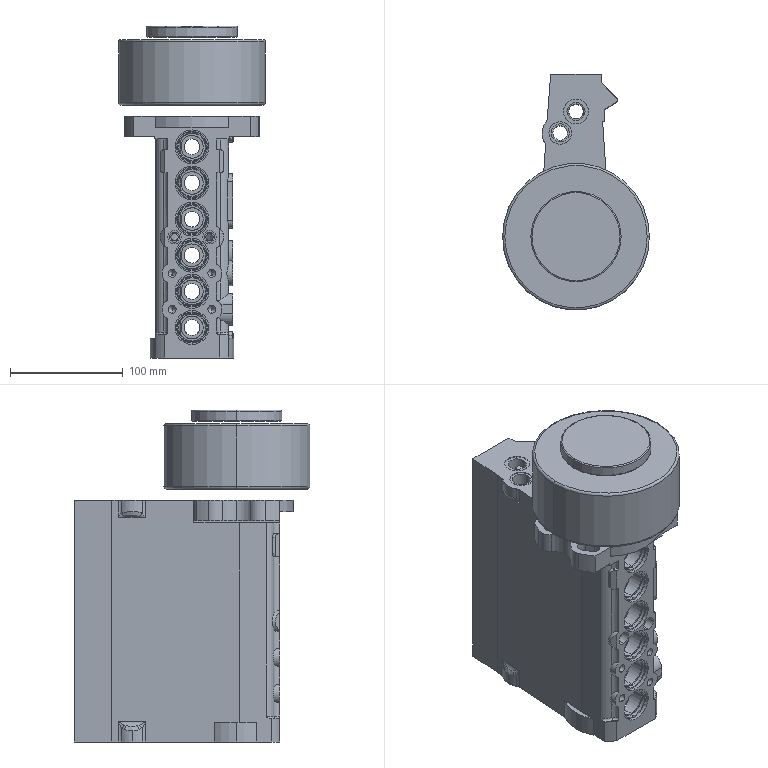Part | SolidWorks | features BaseBody 3 | 3 solids | 994 faces | box 130 x 209 x 294 mm | volume 2004246 mm3 | cylinder 473 | plane 357 | torus 57 | spline 51 | cone 48 | sphere 8 | commonest cylinder face diameters 20 x28 6 x26 6.596 x24 13 x24 14.5 x24 24 x24